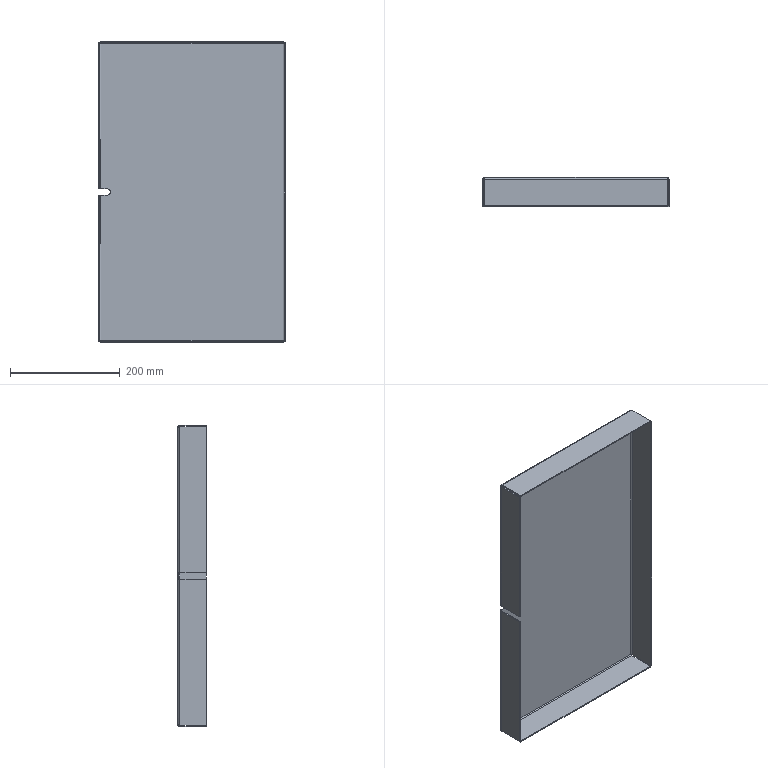Part | STEP file | Produce dryer line heating fan-OVEN-455 | 1 solid | 46 faces | box 340 x 52 x 550 mm | volume 543570 mm3 | plane 27 | cylinder 11 | spline 8 | commonest cylinder face diameters 4 x5 8 x5 12 x1